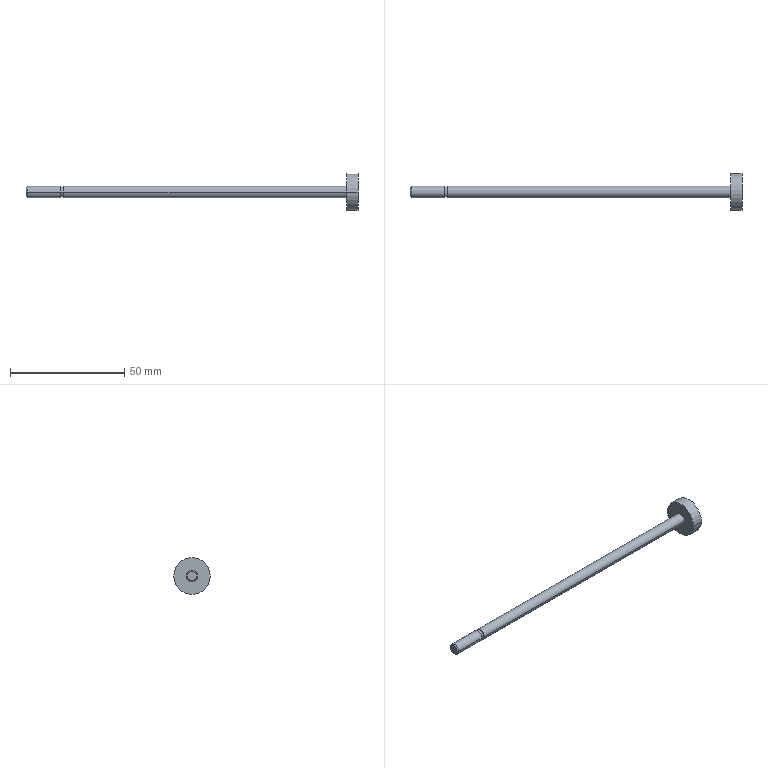Part | SolidWorks | features RefAxis 9, 3DProfileFeature 3, Revolution 1 | 1 solid | 15 faces | box 145.5 x 16 x 16 mm | volume 3753 mm3 | cylinder 8 | plane 5 | cone 2 | commonest cylinder face diameters 5 x4 4.134 x2 16 x2
STEP:
#1=CARTESIAN_POINT('',(145.5,-8.,0.));
#2=VERTEX_POINT('',#1);
#3=CARTESIAN_POINT('',(145.5,8.,0.));
#4=VERTEX_POINT('',#3);
#5=CARTESIAN_POINT('',(145.5,0.,0.));
#6=DIRECTION('',(-1.,0.,0.));
#7=DIRECTION('',(0.,-1.,0.));
#8=AXIS2_PLACEMENT_3D('',#5,#6,#7);
#9=CIRCLE('',#8,8.);
#10=EDGE_CURVE('',#2,#4,#9,.T.);
#11=ORIENTED_EDGE('',*,*,#10,.T.);
#12=CARTESIAN_POINT('',(140.5,8.,0.));
#13=VERTEX_POINT('',#12);
#14=CARTESIAN_POINT('',(145.5,8.,0.));
#15=DIRECTION('',(-1.,0.,0.));
#16=VECTOR('',#15,1000.);
#17=LINE('',#14,#16);
#18=EDGE_CURVE('',#4,#13,#17,.T.);
#19=ORIENTED_EDGE('',*,*,#18,.T.);
#20=CARTESIAN_POINT('',(140.5,-8.,0.));
#21=VERTEX_POINT('',#20);
#22=CARTESIAN_POINT('',(140.5,0.,0.));
#23=DIRECTION('',(-1.,0.,0.));
#24=DIRECTION('',(0.,-1.,0.));
#25=AXIS2_PLACEMENT_3D('',#22,#23,#24);
#26=CIRCLE('',#25,8.);
#27=EDGE_CURVE('',#21,#13,#26,.T.);
#28=ORIENTED_EDGE('',*,*,#27,.F.);
#29=CARTESIAN_POINT('',(145.5,-8.,0.));
#30=DIRECTION('',(-1.,0.,0.));
#31=VECTOR('',#30,1000.);
#32=LINE('',#29,#31);
#33=EDGE_CURVE('',#2,#21,#32,.T.);
#34=ORIENTED_EDGE('',*,*,#33,.F.);
#35=EDGE_LOOP('',(#11,#19,#28,#34));
#36=FACE_OUTER_BOUND('',#35,.T.);
#37=CARTESIAN_POINT('',(145.5,0.,0.));
#38=DIRECTION('',(-1.,0.,0.));
#39=DIRECTION('',(0.,-1.,0.));
#40=AXIS2_PLACEMENT_3D('',#37,#38,#39);
#41=CYLINDRICAL_SURFACE('',#40,8.);
#42=ADVANCED_FACE('',(#36),#41,.T.);
#43=CARTESIAN_POINT('',(140.5,-2.5,0.));
#44=VERTEX_POINT('',#43);
#45=CARTESIAN_POINT('',(140.5,2.5,0.));
#46=VERTEX_POINT('',#45);
#47=CARTESIAN_POINT('',(140.5,0.,0.));
#48=DIRECTION('',(-1.,0.,0.));
#49=DIRECTION('',(0.,-1.,0.));
#50=AXIS2_PLACEMENT_3D('',#47,#48,#49);
#51=CIRCLE('',#50,2.5);
#52=EDGE_CURVE('',#44,#46,#51,.T.);
#53=ORIENTED_EDGE('',*,*,#52,.T.);
#54=CARTESIAN_POINT('',(16.5,2.5,0.));
#55=VERTEX_POINT('',#54);
#56=CARTESIAN_POINT('',(145.5,2.5,0.));
#57=DIRECTION('',(-1.,0.,0.));
#58=VECTOR('',#57,1000.);
#59=LINE('',#56,#58);
#60=EDGE_CURVE('',#46,#55,#59,.T.);
#61=ORIENTED_EDGE('',*,*,#60,.T.);
#62=CARTESIAN_POINT('',(16.5,-2.5,0.));
#63=VERTEX_POINT('',#62);
#64=CARTESIAN_POINT('',(16.5,0.,0.));
#65=DIRECTION('',(-1.,0.,0.));
#66=DIRECTION('',(0.,-1.,0.));
#67=AXIS2_PLACEMENT_3D('',#64,#65,#66);
#68=CIRCLE('',#67,2.5);
#69=EDGE_CURVE('',#63,#55,#68,.T.);
#70=ORIENTED_EDGE('',*,*,#69,.F.);
#71=CARTESIAN_POINT('',(145.5,-2.5,0.));
#72=DIRECTION('',(-1.,0.,0.));
#73=VECTOR('',#72,1000.);
#74=LINE('',#71,#73);
#75=EDGE_CURVE('',#44,#63,#74,.T.);
#76=ORIENTED_EDGE('',*,*,#75,.F.);
#77=EDGE_LOOP('',(#53,#61,#70,#76));
#78=FACE_OUTER_BOUND('',#77,.T.);
#79=CARTESIAN_POINT('',(145.5,0.,0.));
#80=DIRECTION('',(-1.,0.,0.));
#81=DIRECTION('',(0.,-1.,0.));
#82=AXIS2_PLACEMENT_3D('',#79,#80,#81);
#83=CYLINDRICAL_SURFACE('',#82,2.5);
#84=ADVANCED_FACE('',(#78),#83,.T.);
#85=CARTESIAN_POINT('',(16.5,-2.067,0.));
#86=VERTEX_POINT('',#85);
#87=CARTESIAN_POINT('',(16.5,2.067,0.));
#88=VERTEX_POINT('',#87);
#89=CARTESIAN_POINT('',(16.5,0.,0.));
#90=DIRECTION('',(-1.,0.,0.));
#91=DIRECTION('',(0.,-1.,0.));
#92=AXIS2_PLACEMENT_3D('',#89,#90,#91);
#93=CIRCLE('',#92,2.067);
#94=EDGE_CURVE('',#86,#88,#93,.T.);
#95=ORIENTED_EDGE('',*,*,#94,.T.);
#96=CARTESIAN_POINT('',(15.,2.067,0.));
#97=VERTEX_POINT('',#96);
#98=CARTESIAN_POINT('',(145.5,2.067,0.));
#99=DIRECTION('',(-1.,0.,0.));
#100=VECTOR('',#99,1000.);
#101=LINE('',#98,#100);
#102=EDGE_CURVE('',#88,#97,#101,.T.);
#103=ORIENTED_EDGE('',*,*,#102,.T.);
#104=CARTESIAN_POINT('',(15.,-2.067,0.));
#105=VERTEX_POINT('',#104);
#106=CARTESIAN_POINT('',(15.,0.,0.));
#107=DIRECTION('',(-1.,0.,0.));
#108=DIRECTION('',(0.,-1.,0.));
#109=AXIS2_PLACEMENT_3D('',#106,#107,#108);
#110=CIRCLE('',#109,2.067);
#111=EDGE_CURVE('',#105,#97,#110,.T.);
#112=ORIENTED_EDGE('',*,*,#111,.F.);
#113=CARTESIAN_POINT('',(145.5,-2.067,0.));
#114=DIRECTION('',(-1.,0.,0.));
#115=VECTOR('',#114,1000.);
#116=LINE('',#113,#115);
#117=EDGE_CURVE('',#86,#105,#116,.T.);
#118=ORIENTED_EDGE('',*,*,#117,.F.);
#119=EDGE_LOOP('',(#95,#103,#112,#118));
#120=FACE_OUTER_BOUND('',#119,.T.);
#121=CARTESIAN_POINT('',(145.5,0.,0.));
#122=DIRECTION('',(-1.,0.,0.));
#123=DIRECTION('',(0.,-1.,0.));
#124=AXIS2_PLACEMENT_3D('',#121,#122,#123);
#125=CYLINDRICAL_SURFACE('',#124,2.067);
#126=ADVANCED_FACE('',(#120),#125,.T.);
#127=CARTESIAN_POINT('',(15.,-2.5,0.));
#128=VERTEX_POINT('',#127);
#129=CARTESIAN_POINT('',(15.,2.5,0.));
#130=VERTEX_POINT('',#129);
#131=CARTESIAN_POINT('',(15.,0.,0.));
#132=DIRECTION('',(-1.,0.,0.));
#133=DIRECTION('',(0.,-1.,0.));
#134=AXIS2_PLACEMENT_3D('',#131,#132,#133);
#135=CIRCLE('',#134,2.5);
#136=EDGE_CURVE('',#128,#130,#135,.T.);
#137=ORIENTED_EDGE('',*,*,#136,.T.);
#138=CARTESIAN_POINT('',(0.4905,2.5,0.));
#139=VERTEX_POINT('',#138);
#140=CARTESIAN_POINT('',(145.5,2.5,0.));
#141=DIRECTION('',(-1.,0.,0.));
#142=VECTOR('',#141,1000.);
#143=LINE('',#140,#142);
#144=EDGE_CURVE('',#130,#139,#143,.T.);
#145=ORIENTED_EDGE('',*,*,#144,.T.);
#146=CARTESIAN_POINT('',(0.4905,-2.5,0.));
#147=VERTEX_POINT('',#146);
#148=CARTESIAN_POINT('',(0.4905,0.,0.));
#149=DIRECTION('',(-1.,0.,0.));
#150=DIRECTION('',(0.,-1.,0.));
#151=AXIS2_PLACEMENT_3D('',#148,#149,#150);
#152=CIRCLE('',#151,2.5);
#153=EDGE_CURVE('',#147,#139,#152,.T.);
#154=ORIENTED_EDGE('',*,*,#153,.F.);
#155=CARTESIAN_POINT('',(145.5,-2.5,0.));
#156=DIRECTION('',(-1.,0.,0.));
#157=VECTOR('',#156,1000.);
#158=LINE('',#155,#157);
#159=EDGE_CURVE('',#128,#147,#158,.T.);
#160=ORIENTED_EDGE('',*,*,#159,.F.);
#161=EDGE_LOOP('',(#137,#145,#154,#160));
#162=FACE_OUTER_BOUND('',#161,.T.);
#163=CARTESIAN_POINT('',(145.5,0.,0.));
#164=DIRECTION('',(-1.,0.,0.));
#165=DIRECTION('',(0.,-1.,0.));
#166=AXIS2_PLACEMENT_3D('',#163,#164,#165);
#167=CYLINDRICAL_SURFACE('',#166,2.5);
#168=ADVANCED_FACE('',(#162),#167,.T.);
#169=CARTESIAN_POINT('',(0.,-2.01,0.));
#170=VERTEX_POINT('',#169);
#171=CARTESIAN_POINT('',(0.,2.01,0.));
#172=VERTEX_POINT('',#171);
#173=CARTESIAN_POINT('',(0.,0.,0.));
#174=DIRECTION('',(-1.,0.,0.));
#175=DIRECTION('',(0.,-1.,0.));
#176=AXIS2_PLACEMENT_3D('',#173,#174,#175);
#177=CIRCLE('',#176,2.01);
#178=EDGE_CURVE('',#170,#172,#177,.T.);
#179=ORIENTED_EDGE('',*,*,#178,.F.);
#180=CARTESIAN_POINT('',(0.4905,-2.5,0.));
#181=DIRECTION('',(0.7071,-0.7071,0.));
#182=VECTOR('',#181,1000.);
#183=LINE('',#180,#182);
#184=EDGE_CURVE('',#170,#147,#183,.T.);
#185=ORIENTED_EDGE('',*,*,#184,.T.);
#186=ORIENTED_EDGE('',*,*,#153,.T.);
#187=CARTESIAN_POINT('',(0.4905,2.5,0.));
#188=DIRECTION('',(0.7071,0.7071,0.));
#189=VECTOR('',#188,1000.);
#190=LINE('',#187,#189);
#191=EDGE_CURVE('',#172,#139,#190,.T.);
#192=ORIENTED_EDGE('',*,*,#191,.F.);
#193=EDGE_LOOP('',(#179,#185,#186,#192));
#194=FACE_OUTER_BOUND('',#193,.T.);
#195=CARTESIAN_POINT('',(0.4905,0.,0.));
#196=DIRECTION('',(1.,0.,0.));
#197=DIRECTION('',(0.,1.,0.));
#198=AXIS2_PLACEMENT_3D('',#195,#196,#197);
#199=CONICAL_SURFACE('',#198,2.5,0.7854);
#200=ADVANCED_FACE('',(#194),#199,.T.);
#201=CARTESIAN_POINT('',(0.,0.,0.));
#202=DIRECTION('',(-1.,0.,0.));
#203=DIRECTION('',(0.,-1.,0.));
#204=AXIS2_PLACEMENT_3D('',#201,#202,#203);
#205=CIRCLE('',#204,2.01);
#206=EDGE_CURVE('',#172,#170,#205,.T.);
#207=ORIENTED_EDGE('',*,*,#206,.T.);
#208=ORIENTED_EDGE('',*,*,#178,.T.);
#209=EDGE_LOOP('',(#207,#208));
#210=FACE_OUTER_BOUND('',#209,.T.);
#211=CARTESIAN_POINT('',(0.,0.,0.));
#212=DIRECTION('',(1.,0.,0.));
#213=DIRECTION('',(0.,1.,0.));
#214=AXIS2_PLACEMENT_3D('',#211,#212,#213);
#215=PLANE('',#214);
#216=ADVANCED_FACE('',(#210),#215,.F.);
#217=ORIENTED_EDGE('',*,*,#184,.F.);
#218=ORIENTED_EDGE('',*,*,#206,.F.);
#219=ORIENTED_EDGE('',*,*,#191,.T.);
#220=CARTESIAN_POINT('',(0.4905,0.,0.));
#221=DIRECTION('',(-1.,0.,0.));
#222=DIRECTION('',(0.,-1.,0.));
#223=AXIS2_PLACEMENT_3D('',#220,#221,#222);
#224=CIRCLE('',#223,2.5);
#225=EDGE_CURVE('',#139,#147,#224,.T.);
#226=ORIENTED_EDGE('',*,*,#225,.T.);
#227=EDGE_LOOP('',(#217,#218,#219,#226));
#228=FACE_OUTER_BOUND('',#227,.T.);
#229=CARTESIAN_POINT('',(0.4905,0.,0.));
#230=DIRECTION('',(1.,0.,0.));
#231=DIRECTION('',(0.,1.,0.));
#232=AXIS2_PLACEMENT_3D('',#229,#230,#231);
#233=CONICAL_SURFACE('',#232,2.5,0.7854);
#234=ADVANCED_FACE('',(#228),#233,.T.);
#235=ORIENTED_EDGE('',*,*,#144,.F.);
#236=CARTESIAN_POINT('',(15.,0.,0.));
#237=DIRECTION('',(-1.,0.,0.));
#238=DIRECTION('',(0.,-1.,0.));
#239=AXIS2_PLACEMENT_3D('',#236,#237,#238);
#240=CIRCLE('',#239,2.5);
#241=EDGE_CURVE('',#130,#128,#240,.T.);
#242=ORIENTED_EDGE('',*,*,#241,.T.);
#243=ORIENTED_EDGE('',*,*,#159,.T.);
#244=ORIENTED_EDGE('',*,*,#225,.F.);
#245=EDGE_LOOP('',(#235,#242,#243,#244));
#246=FACE_OUTER_BOUND('',#245,.T.);
#247=CARTESIAN_POINT('',(145.5,0.,0.));
#248=DIRECTION('',(-1.,0.,0.));
#249=DIRECTION('',(0.,-1.,0.));
#250=AXIS2_PLACEMENT_3D('',#247,#248,#249);
#251=CYLINDRICAL_SURFACE('',#250,2.5);
#252=ADVANCED_FACE('',(#246),#251,.T.);
#253=ORIENTED_EDGE('',*,*,#136,.F.);
#254=ORIENTED_EDGE('',*,*,#241,.F.);
#255=EDGE_LOOP('',(#253,#254));
#256=FACE_OUTER_BOUND('',#255,.T.);
#257=ORIENTED_EDGE('',*,*,#111,.T.);
#258=CARTESIAN_POINT('',(15.,0.,0.));
#259=DIRECTION('',(-1.,0.,0.));
#260=DIRECTION('',(0.,-1.,0.));
#261=AXIS2_PLACEMENT_3D('',#258,#259,#260);
#262=CIRCLE('',#261,2.067);
#263=EDGE_CURVE('',#97,#105,#262,.T.);
#264=ORIENTED_EDGE('',*,*,#263,.T.);
#265=EDGE_LOOP('',(#257,#264));
#266=FACE_BOUND('',#265,.T.);
#267=CARTESIAN_POINT('',(15.,2.5,0.));
#268=DIRECTION('',(-1.,0.,0.));
#269=DIRECTION('',(0.,-1.,0.));
#270=AXIS2_PLACEMENT_3D('',#267,#268,#269);
#271=PLANE('',#270);
#272=ADVANCED_FACE('',(#256,#266),#271,.F.);
#273=ORIENTED_EDGE('',*,*,#102,.F.);
#274=CARTESIAN_POINT('',(16.5,0.,0.));
#275=DIRECTION('',(-1.,0.,0.));
#276=DIRECTION('',(0.,-1.,0.));
#277=AXIS2_PLACEMENT_3D('',#274,#275,#276);
#278=CIRCLE('',#277,2.067);
#279=EDGE_CURVE('',#88,#86,#278,.T.);
#280=ORIENTED_EDGE('',*,*,#279,.T.);
#281=ORIENTED_EDGE('',*,*,#117,.T.);
#282=ORIENTED_EDGE('',*,*,#263,.F.);
#283=EDGE_LOOP('',(#273,#280,#281,#282));
#284=FACE_OUTER_BOUND('',#283,.T.);
#285=CARTESIAN_POINT('',(145.5,0.,0.));
#286=DIRECTION('',(-1.,0.,0.));
#287=DIRECTION('',(0.,-1.,0.));
#288=AXIS2_PLACEMENT_3D('',#285,#286,#287);
#289=CYLINDRICAL_SURFACE('',#288,2.067);
#290=ADVANCED_FACE('',(#284),#289,.T.);
#291=ORIENTED_EDGE('',*,*,#94,.F.);
#292=ORIENTED_EDGE('',*,*,#279,.F.);
#293=EDGE_LOOP('',(#291,#292));
#294=FACE_BOUND('',#293,.T.);
#295=ORIENTED_EDGE('',*,*,#69,.T.);
#296=CARTESIAN_POINT('',(16.5,0.,0.));
#297=DIRECTION('',(-1.,0.,0.));
#298=DIRECTION('',(0.,-1.,0.));
#299=AXIS2_PLACEMENT_3D('',#296,#297,#298);
#300=CIRCLE('',#299,2.5);
#301=EDGE_CURVE('',#55,#63,#300,.T.);
#302=ORIENTED_EDGE('',*,*,#301,.T.);
#303=EDGE_LOOP('',(#295,#302));
#304=FACE_OUTER_BOUND('',#303,.T.);
#305=CARTESIAN_POINT('',(16.5,2.067,0.));
#306=DIRECTION('',(1.,0.,0.));
#307=DIRECTION('',(0.,1.,0.));
#308=AXIS2_PLACEMENT_3D('',#305,#306,#307);
#309=PLANE('',#308);
#310=ADVANCED_FACE('',(#294,#304),#309,.F.);
#311=ORIENTED_EDGE('',*,*,#60,.F.);
#312=CARTESIAN_POINT('',(140.5,0.,0.));
#313=DIRECTION('',(-1.,0.,0.));
#314=DIRECTION('',(0.,-1.,0.));
#315=AXIS2_PLACEMENT_3D('',#312,#313,#314);
#316=CIRCLE('',#315,2.5);
#317=EDGE_CURVE('',#46,#44,#316,.T.);
#318=ORIENTED_EDGE('',*,*,#317,.T.);
#319=ORIENTED_EDGE('',*,*,#75,.T.);
#320=ORIENTED_EDGE('',*,*,#301,.F.);
#321=EDGE_LOOP('',(#311,#318,#319,#320));
#322=FACE_OUTER_BOUND('',#321,.T.);
#323=CARTESIAN_POINT('',(145.5,0.,0.));
#324=DIRECTION('',(-1.,0.,0.));
#325=DIRECTION('',(0.,-1.,0.));
#326=AXIS2_PLACEMENT_3D('',#323,#324,#325);
#327=CYLINDRICAL_SURFACE('',#326,2.5);
#328=ADVANCED_FACE('',(#322),#327,.T.);
#329=ORIENTED_EDGE('',*,*,#52,.F.);
#330=ORIENTED_EDGE('',*,*,#317,.F.);
#331=EDGE_LOOP('',(#329,#330));
#332=FACE_BOUND('',#331,.T.);
#333=ORIENTED_EDGE('',*,*,#27,.T.);
#334=CARTESIAN_POINT('',(140.5,0.,0.));
#335=DIRECTION('',(-1.,0.,0.));
#336=DIRECTION('',(0.,-1.,0.));
#337=AXIS2_PLACEMENT_3D('',#334,#335,#336);
#338=CIRCLE('',#337,8.);
#339=EDGE_CURVE('',#13,#21,#338,.T.);
#340=ORIENTED_EDGE('',*,*,#339,.T.);
#341=EDGE_LOOP('',(#333,#340));
#342=FACE_OUTER_BOUND('',#341,.T.);
#343=CARTESIAN_POINT('',(140.5,2.5,0.));
#344=DIRECTION('',(1.,0.,0.));
#345=DIRECTION('',(0.,1.,0.));
#346=AXIS2_PLACEMENT_3D('',#343,#344,#345);
#347=PLANE('',#346);
#348=ADVANCED_FACE('',(#332,#342),#347,.F.);
#349=ORIENTED_EDGE('',*,*,#18,.F.);
#350=CARTESIAN_POINT('',(145.5,0.,0.));
#351=DIRECTION('',(-1.,0.,0.));
#352=DIRECTION('',(0.,-1.,0.));
#353=AXIS2_PLACEMENT_3D('',#350,#351,#352);
#354=CIRCLE('',#353,8.);
#355=EDGE_CURVE('',#4,#2,#354,.T.);
#356=ORIENTED_EDGE('',*,*,#355,.T.);
#357=ORIENTED_EDGE('',*,*,#33,.T.);
#358=ORIENTED_EDGE('',*,*,#339,.F.);
#359=EDGE_LOOP('',(#349,#356,#357,#358));
#360=FACE_OUTER_BOUND('',#359,.T.);
#361=CARTESIAN_POINT('',(145.5,0.,0.));
#362=DIRECTION('',(-1.,0.,0.));
#363=DIRECTION('',(0.,-1.,0.));
#364=AXIS2_PLACEMENT_3D('',#361,#362,#363);
#365=CYLINDRICAL_SURFACE('',#364,8.);
#366=ADVANCED_FACE('',(#360),#365,.T.);
#367=ORIENTED_EDGE('',*,*,#10,.F.);
#368=ORIENTED_EDGE('',*,*,#355,.F.);
#369=EDGE_LOOP('',(#367,#368));
#370=FACE_OUTER_BOUND('',#369,.T.);
#371=CARTESIAN_POINT('',(145.5,8.,0.));
#372=DIRECTION('',(-1.,0.,0.));
#373=DIRECTION('',(0.,-1.,0.));
#374=AXIS2_PLACEMENT_3D('',#371,#372,#373);
#375=PLANE('',#374);
#376=ADVANCED_FACE('',(#370),#375,.F.);
#377=CLOSED_SHELL('',(#42,#84,#126,#168,#200,#216,#234,#252,#272,#290,#310,#328,#348,#366,#376));
#378=MANIFOLD_SOLID_BREP('',#377);
#379=CARTESIAN_POINT('',(0.,0.,0.));
#380=DIRECTION('',(0.,0.,1.));
#381=DIRECTION('',(1.,0.,0.));
#382=AXIS2_PLACEMENT_3D('',#379,#380,#381);
#383=(LENGTH_UNIT()NAMED_UNIT(*)SI_UNIT(.MILLI.,.METRE.));
#384=UNCERTAINTY_MEASURE_WITH_UNIT(LENGTH_MEASURE(0.00001),#383,'','');
#385=(NAMED_UNIT(*)PLANE_ANGLE_UNIT()SI_UNIT($,.RADIAN.));
#386=(NAMED_UNIT(*)SI_UNIT($,.STERADIAN.)SOLID_ANGLE_UNIT());
#387=(GEOMETRIC_REPRESENTATION_CONTEXT(3)GLOBAL_UNCERTAINTY_ASSIGNED_CONTEXT((#384))GLOBAL_UNIT_ASSIGNED_CONTEXT((#383,#385,#386))REPRESENTATION_CONTEXT('',''));
#388=ADVANCED_BREP_SHAPE_REPRESENTATION('',(#378,#382),#387);